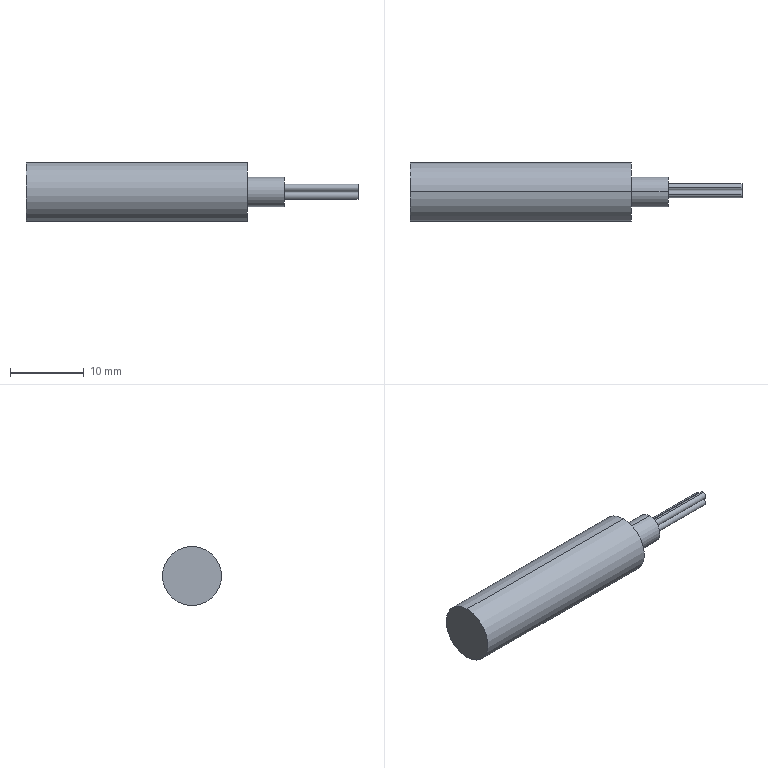Part | STEP file | Sensors | 1 solid | 16 faces | box 45 x 8 x 8 mm | volume 1594 mm3 | cylinder 10 | plane 6 | commonest cylinder face diameters 1 x6 4 x2 8 x2
STEP:
#1=CARTESIAN_POINT('',(34.739,-0.2752,0.03902));
#2=VERTEX_POINT('',#1);
#3=CARTESIAN_POINT('',(34.739,-0.2752,1.039));
#4=VERTEX_POINT('',#3);
#5=CARTESIAN_POINT('',(34.739,-0.2752,0.539));
#6=DIRECTION('',(1.,0.,0.));
#7=DIRECTION('',(0.,0.,-1.));
#8=AXIS2_PLACEMENT_3D('',#5,#6,#7);
#9=CIRCLE('',#8,0.5);
#10=EDGE_CURVE('',#2,#4,#9,.T.);
#11=ORIENTED_EDGE('',*,*,#10,.F.);
#12=CARTESIAN_POINT('',(24.739,-0.2752,0.03902));
#13=VERTEX_POINT('',#12);
#14=CARTESIAN_POINT('',(34.739,-0.2752,0.03902));
#15=DIRECTION('',(-1.,0.,0.));
#16=VECTOR('',#15,1000.);
#17=LINE('',#14,#16);
#18=EDGE_CURVE('',#2,#13,#17,.T.);
#19=ORIENTED_EDGE('',*,*,#18,.T.);
#20=CARTESIAN_POINT('',(24.739,-0.2752,1.039));
#21=VERTEX_POINT('',#20);
#22=CARTESIAN_POINT('',(24.739,-0.2752,0.539));
#23=DIRECTION('',(1.,0.,0.));
#24=DIRECTION('',(0.,0.,-1.));
#25=AXIS2_PLACEMENT_3D('',#22,#23,#24);
#26=CIRCLE('',#25,0.5);
#27=EDGE_CURVE('',#13,#21,#26,.T.);
#28=ORIENTED_EDGE('',*,*,#27,.T.);
#29=CARTESIAN_POINT('',(34.739,-0.2752,1.039));
#30=DIRECTION('',(-1.,0.,0.));
#31=VECTOR('',#30,1000.);
#32=LINE('',#29,#31);
#33=EDGE_CURVE('',#4,#21,#32,.T.);
#34=ORIENTED_EDGE('',*,*,#33,.F.);
#35=EDGE_LOOP('',(#11,#19,#28,#34));
#36=FACE_OUTER_BOUND('',#35,.T.);
#37=CARTESIAN_POINT('',(34.739,-0.2752,0.539));
#38=DIRECTION('',(-1.,0.,0.));
#39=DIRECTION('',(0.,0.,1.));
#40=AXIS2_PLACEMENT_3D('',#37,#38,#39);
#41=CYLINDRICAL_SURFACE('',#40,0.5);
#42=ADVANCED_FACE('',(#36),#41,.T.);
#43=CARTESIAN_POINT('',(34.739,-0.2752,-1.016));
#44=VERTEX_POINT('',#43);
#45=CARTESIAN_POINT('',(34.739,-0.2752,-0.01608));
#46=VERTEX_POINT('',#45);
#47=CARTESIAN_POINT('',(34.739,-0.2752,-0.5161));
#48=DIRECTION('',(1.,0.,0.));
#49=DIRECTION('',(0.,0.,-1.));
#50=AXIS2_PLACEMENT_3D('',#47,#48,#49);
#51=CIRCLE('',#50,0.5);
#52=EDGE_CURVE('',#44,#46,#51,.T.);
#53=ORIENTED_EDGE('',*,*,#52,.F.);
#54=CARTESIAN_POINT('',(24.739,-0.2752,-1.016));
#55=VERTEX_POINT('',#54);
#56=CARTESIAN_POINT('',(34.739,-0.2752,-1.016));
#57=DIRECTION('',(-1.,0.,0.));
#58=VECTOR('',#57,1000.);
#59=LINE('',#56,#58);
#60=EDGE_CURVE('',#44,#55,#59,.T.);
#61=ORIENTED_EDGE('',*,*,#60,.T.);
#62=CARTESIAN_POINT('',(24.739,-0.2752,-0.01608));
#63=VERTEX_POINT('',#62);
#64=CARTESIAN_POINT('',(24.739,-0.2752,-0.5161));
#65=DIRECTION('',(1.,0.,0.));
#66=DIRECTION('',(0.,0.,-1.));
#67=AXIS2_PLACEMENT_3D('',#64,#65,#66);
#68=CIRCLE('',#67,0.5);
#69=EDGE_CURVE('',#55,#63,#68,.T.);
#70=ORIENTED_EDGE('',*,*,#69,.T.);
#71=CARTESIAN_POINT('',(34.739,-0.2752,-0.01608));
#72=DIRECTION('',(-1.,0.,0.));
#73=VECTOR('',#72,1000.);
#74=LINE('',#71,#73);
#75=EDGE_CURVE('',#46,#63,#74,.T.);
#76=ORIENTED_EDGE('',*,*,#75,.F.);
#77=EDGE_LOOP('',(#53,#61,#70,#76));
#78=FACE_OUTER_BOUND('',#77,.T.);
#79=CARTESIAN_POINT('',(34.739,-0.2752,-0.5161));
#80=DIRECTION('',(-1.,0.,0.));
#81=DIRECTION('',(0.,0.,1.));
#82=AXIS2_PLACEMENT_3D('',#79,#80,#81);
#83=CYLINDRICAL_SURFACE('',#82,0.5);
#84=ADVANCED_FACE('',(#78),#83,.T.);
#85=CARTESIAN_POINT('',(34.739,0.6078,-0.5));
#86=VERTEX_POINT('',#85);
#87=CARTESIAN_POINT('',(34.739,0.6078,0.5));
#88=VERTEX_POINT('',#87);
#89=CARTESIAN_POINT('',(34.739,0.6078,0.));
#90=DIRECTION('',(1.,0.,0.));
#91=DIRECTION('',(0.,0.,-1.));
#92=AXIS2_PLACEMENT_3D('',#89,#90,#91);
#93=CIRCLE('',#92,0.5);
#94=EDGE_CURVE('',#86,#88,#93,.T.);
#95=ORIENTED_EDGE('',*,*,#94,.F.);
#96=CARTESIAN_POINT('',(24.739,0.6078,-0.5));
#97=VERTEX_POINT('',#96);
#98=CARTESIAN_POINT('',(34.739,0.6078,-0.5));
#99=DIRECTION('',(-1.,0.,0.));
#100=VECTOR('',#99,1000.);
#101=LINE('',#98,#100);
#102=EDGE_CURVE('',#86,#97,#101,.T.);
#103=ORIENTED_EDGE('',*,*,#102,.T.);
#104=CARTESIAN_POINT('',(24.739,0.6078,0.5));
#105=VERTEX_POINT('',#104);
#106=CARTESIAN_POINT('',(24.739,0.6078,0.));
#107=DIRECTION('',(1.,0.,0.));
#108=DIRECTION('',(0.,0.,-1.));
#109=AXIS2_PLACEMENT_3D('',#106,#107,#108);
#110=CIRCLE('',#109,0.5);
#111=EDGE_CURVE('',#97,#105,#110,.T.);
#112=ORIENTED_EDGE('',*,*,#111,.T.);
#113=CARTESIAN_POINT('',(34.739,0.6078,0.5));
#114=DIRECTION('',(-1.,0.,0.));
#115=VECTOR('',#114,1000.);
#116=LINE('',#113,#115);
#117=EDGE_CURVE('',#88,#105,#116,.T.);
#118=ORIENTED_EDGE('',*,*,#117,.F.);
#119=EDGE_LOOP('',(#95,#103,#112,#118));
#120=FACE_OUTER_BOUND('',#119,.T.);
#121=CARTESIAN_POINT('',(34.739,0.6078,0.));
#122=DIRECTION('',(-1.,0.,0.));
#123=DIRECTION('',(0.,0.,1.));
#124=AXIS2_PLACEMENT_3D('',#121,#122,#123);
#125=CYLINDRICAL_SURFACE('',#124,0.5);
#126=ADVANCED_FACE('',(#120),#125,.T.);
#127=CARTESIAN_POINT('',(24.739,0.,-2.));
#128=VERTEX_POINT('',#127);
#129=CARTESIAN_POINT('',(24.739,0.,2.));
#130=VERTEX_POINT('',#129);
#131=CARTESIAN_POINT('',(24.739,0.,0.));
#132=DIRECTION('',(1.,0.,0.));
#133=DIRECTION('',(0.,0.,-1.));
#134=AXIS2_PLACEMENT_3D('',#131,#132,#133);
#135=CIRCLE('',#134,2.);
#136=EDGE_CURVE('',#128,#130,#135,.T.);
#137=ORIENTED_EDGE('',*,*,#136,.F.);
#138=CARTESIAN_POINT('',(19.739,0.,-2.));
#139=VERTEX_POINT('',#138);
#140=CARTESIAN_POINT('',(24.739,0.,-2.));
#141=DIRECTION('',(-1.,0.,0.));
#142=VECTOR('',#141,1000.);
#143=LINE('',#140,#142);
#144=EDGE_CURVE('',#128,#139,#143,.T.);
#145=ORIENTED_EDGE('',*,*,#144,.T.);
#146=CARTESIAN_POINT('',(19.739,0.,2.));
#147=VERTEX_POINT('',#146);
#148=CARTESIAN_POINT('',(19.739,0.,0.));
#149=DIRECTION('',(1.,0.,0.));
#150=DIRECTION('',(0.,0.,-1.));
#151=AXIS2_PLACEMENT_3D('',#148,#149,#150);
#152=CIRCLE('',#151,2.);
#153=EDGE_CURVE('',#139,#147,#152,.T.);
#154=ORIENTED_EDGE('',*,*,#153,.T.);
#155=CARTESIAN_POINT('',(24.739,0.,2.));
#156=DIRECTION('',(-1.,0.,0.));
#157=VECTOR('',#156,1000.);
#158=LINE('',#155,#157);
#159=EDGE_CURVE('',#130,#147,#158,.T.);
#160=ORIENTED_EDGE('',*,*,#159,.F.);
#161=EDGE_LOOP('',(#137,#145,#154,#160));
#162=FACE_OUTER_BOUND('',#161,.T.);
#163=CARTESIAN_POINT('',(24.739,0.,0.));
#164=DIRECTION('',(-1.,0.,0.));
#165=DIRECTION('',(0.,0.,1.));
#166=AXIS2_PLACEMENT_3D('',#163,#164,#165);
#167=CYLINDRICAL_SURFACE('',#166,2.);
#168=ADVANCED_FACE('',(#162),#167,.T.);
#169=CARTESIAN_POINT('',(19.739,0.,4.));
#170=VERTEX_POINT('',#169);
#171=CARTESIAN_POINT('',(19.739,0.,-4.));
#172=VERTEX_POINT('',#171);
#173=CARTESIAN_POINT('',(19.739,0.,0.));
#174=DIRECTION('',(-1.,0.,0.));
#175=DIRECTION('',(0.,0.,1.));
#176=AXIS2_PLACEMENT_3D('',#173,#174,#175);
#177=CIRCLE('',#176,4.);
#178=EDGE_CURVE('',#170,#172,#177,.T.);
#179=ORIENTED_EDGE('',*,*,#178,.T.);
#180=CARTESIAN_POINT('',(-10.261,0.,-4.));
#181=VERTEX_POINT('',#180);
#182=CARTESIAN_POINT('',(-34.395,0.,-4.));
#183=DIRECTION('',(-1.,0.,0.));
#184=VECTOR('',#183,1000.);
#185=LINE('',#182,#184);
#186=EDGE_CURVE('',#172,#181,#185,.T.);
#187=ORIENTED_EDGE('',*,*,#186,.T.);
#188=CARTESIAN_POINT('',(-10.261,0.,4.));
#189=VERTEX_POINT('',#188);
#190=CARTESIAN_POINT('',(-10.261,0.,0.));
#191=DIRECTION('',(-1.,0.,0.));
#192=DIRECTION('',(0.,0.,1.));
#193=AXIS2_PLACEMENT_3D('',#190,#191,#192);
#194=CIRCLE('',#193,4.);
#195=EDGE_CURVE('',#189,#181,#194,.T.);
#196=ORIENTED_EDGE('',*,*,#195,.F.);
#197=CARTESIAN_POINT('',(-34.395,0.,4.));
#198=DIRECTION('',(-1.,0.,0.));
#199=VECTOR('',#198,1000.);
#200=LINE('',#197,#199);
#201=EDGE_CURVE('',#170,#189,#200,.T.);
#202=ORIENTED_EDGE('',*,*,#201,.F.);
#203=EDGE_LOOP('',(#179,#187,#196,#202));
#204=FACE_OUTER_BOUND('',#203,.T.);
#205=CARTESIAN_POINT('',(-34.395,0.,0.));
#206=DIRECTION('',(-1.,0.,0.));
#207=DIRECTION('',(0.,0.,1.));
#208=AXIS2_PLACEMENT_3D('',#205,#206,#207);
#209=CYLINDRICAL_SURFACE('',#208,4.);
#210=ADVANCED_FACE('',(#204),#209,.T.);
#211=ORIENTED_EDGE('',*,*,#195,.T.);
#212=CARTESIAN_POINT('',(-10.261,0.,0.));
#213=DIRECTION('',(-1.,0.,0.));
#214=DIRECTION('',(0.,0.,1.));
#215=AXIS2_PLACEMENT_3D('',#212,#213,#214);
#216=CIRCLE('',#215,4.);
#217=EDGE_CURVE('',#181,#189,#216,.T.);
#218=ORIENTED_EDGE('',*,*,#217,.T.);
#219=EDGE_LOOP('',(#211,#218));
#220=FACE_OUTER_BOUND('',#219,.T.);
#221=CARTESIAN_POINT('',(-10.261,0.,0.));
#222=DIRECTION('',(1.,0.,0.));
#223=DIRECTION('',(0.,0.,-1.));
#224=AXIS2_PLACEMENT_3D('',#221,#222,#223);
#225=PLANE('',#224);
#226=ADVANCED_FACE('',(#220),#225,.F.);
#227=CARTESIAN_POINT('',(19.739,0.,0.));
#228=DIRECTION('',(1.,0.,0.));
#229=DIRECTION('',(0.,0.,-1.));
#230=AXIS2_PLACEMENT_3D('',#227,#228,#229);
#231=CIRCLE('',#230,2.);
#232=EDGE_CURVE('',#147,#139,#231,.T.);
#233=ORIENTED_EDGE('',*,*,#232,.F.);
#234=ORIENTED_EDGE('',*,*,#153,.F.);
#235=EDGE_LOOP('',(#233,#234));
#236=FACE_BOUND('',#235,.T.);
#237=ORIENTED_EDGE('',*,*,#178,.F.);
#238=CARTESIAN_POINT('',(19.739,0.,0.));
#239=DIRECTION('',(-1.,0.,0.));
#240=DIRECTION('',(0.,0.,1.));
#241=AXIS2_PLACEMENT_3D('',#238,#239,#240);
#242=CIRCLE('',#241,4.);
#243=EDGE_CURVE('',#172,#170,#242,.T.);
#244=ORIENTED_EDGE('',*,*,#243,.F.);
#245=EDGE_LOOP('',(#237,#244));
#246=FACE_OUTER_BOUND('',#245,.T.);
#247=CARTESIAN_POINT('',(19.739,0.,0.));
#248=DIRECTION('',(-1.,0.,0.));
#249=DIRECTION('',(0.,0.,1.));
#250=AXIS2_PLACEMENT_3D('',#247,#248,#249);
#251=PLANE('',#250);
#252=ADVANCED_FACE('',(#236,#246),#251,.F.);
#253=ORIENTED_EDGE('',*,*,#186,.F.);
#254=ORIENTED_EDGE('',*,*,#243,.T.);
#255=ORIENTED_EDGE('',*,*,#201,.T.);
#256=ORIENTED_EDGE('',*,*,#217,.F.);
#257=EDGE_LOOP('',(#253,#254,#255,#256));
#258=FACE_OUTER_BOUND('',#257,.T.);
#259=CARTESIAN_POINT('',(-34.395,0.,0.));
#260=DIRECTION('',(-1.,0.,0.));
#261=DIRECTION('',(0.,0.,1.));
#262=AXIS2_PLACEMENT_3D('',#259,#260,#261);
#263=CYLINDRICAL_SURFACE('',#262,4.);
#264=ADVANCED_FACE('',(#258),#263,.T.);
#265=ORIENTED_EDGE('',*,*,#144,.F.);
#266=CARTESIAN_POINT('',(24.739,0.,0.));
#267=DIRECTION('',(1.,0.,0.));
#268=DIRECTION('',(0.,0.,-1.));
#269=AXIS2_PLACEMENT_3D('',#266,#267,#268);
#270=CIRCLE('',#269,2.);
#271=EDGE_CURVE('',#130,#128,#270,.T.);
#272=ORIENTED_EDGE('',*,*,#271,.F.);
#273=ORIENTED_EDGE('',*,*,#159,.T.);
#274=ORIENTED_EDGE('',*,*,#232,.T.);
#275=EDGE_LOOP('',(#265,#272,#273,#274));
#276=FACE_OUTER_BOUND('',#275,.T.);
#277=CARTESIAN_POINT('',(24.739,0.,0.));
#278=DIRECTION('',(-1.,0.,0.));
#279=DIRECTION('',(0.,0.,1.));
#280=AXIS2_PLACEMENT_3D('',#277,#278,#279);
#281=CYLINDRICAL_SURFACE('',#280,2.);
#282=ADVANCED_FACE('',(#276),#281,.T.);
#283=CARTESIAN_POINT('',(24.739,-0.2752,0.539));
#284=DIRECTION('',(1.,0.,0.));
#285=DIRECTION('',(0.,0.,-1.));
#286=AXIS2_PLACEMENT_3D('',#283,#284,#285);
#287=CIRCLE('',#286,0.5);
#288=EDGE_CURVE('',#21,#13,#287,.T.);
#289=ORIENTED_EDGE('',*,*,#288,.F.);
#290=ORIENTED_EDGE('',*,*,#27,.F.);
#291=EDGE_LOOP('',(#289,#290));
#292=FACE_BOUND('',#291,.T.);
#293=CARTESIAN_POINT('',(24.739,-0.2752,-0.5161));
#294=DIRECTION('',(1.,0.,0.));
#295=DIRECTION('',(0.,0.,-1.));
#296=AXIS2_PLACEMENT_3D('',#293,#294,#295);
#297=CIRCLE('',#296,0.5);
#298=EDGE_CURVE('',#63,#55,#297,.T.);
#299=ORIENTED_EDGE('',*,*,#298,.F.);
#300=ORIENTED_EDGE('',*,*,#69,.F.);
#301=EDGE_LOOP('',(#299,#300));
#302=FACE_BOUND('',#301,.T.);
#303=CARTESIAN_POINT('',(24.739,0.6078,0.));
#304=DIRECTION('',(1.,0.,0.));
#305=DIRECTION('',(0.,0.,-1.));
#306=AXIS2_PLACEMENT_3D('',#303,#304,#305);
#307=CIRCLE('',#306,0.5);
#308=EDGE_CURVE('',#105,#97,#307,.T.);
#309=ORIENTED_EDGE('',*,*,#308,.F.);
#310=ORIENTED_EDGE('',*,*,#111,.F.);
#311=EDGE_LOOP('',(#309,#310));
#312=FACE_BOUND('',#311,.T.);
#313=ORIENTED_EDGE('',*,*,#271,.T.);
#314=ORIENTED_EDGE('',*,*,#136,.T.);
#315=EDGE_LOOP('',(#313,#314));
#316=FACE_OUTER_BOUND('',#315,.T.);
#317=CARTESIAN_POINT('',(24.739,0.,0.));
#318=DIRECTION('',(1.,0.,0.));
#319=DIRECTION('',(0.,0.,-1.));
#320=AXIS2_PLACEMENT_3D('',#317,#318,#319);
#321=PLANE('',#320);
#322=ADVANCED_FACE('',(#292,#302,#312,#316),#321,.T.);
#323=ORIENTED_EDGE('',*,*,#102,.F.);
#324=CARTESIAN_POINT('',(34.739,0.6078,0.));
#325=DIRECTION('',(1.,0.,0.));
#326=DIRECTION('',(0.,0.,-1.));
#327=AXIS2_PLACEMENT_3D('',#324,#325,#326);
#328=CIRCLE('',#327,0.5);
#329=EDGE_CURVE('',#88,#86,#328,.T.);
#330=ORIENTED_EDGE('',*,*,#329,.F.);
#331=ORIENTED_EDGE('',*,*,#117,.T.);
#332=ORIENTED_EDGE('',*,*,#308,.T.);
#333=EDGE_LOOP('',(#323,#330,#331,#332));
#334=FACE_OUTER_BOUND('',#333,.T.);
#335=CARTESIAN_POINT('',(34.739,0.6078,0.));
#336=DIRECTION('',(-1.,0.,0.));
#337=DIRECTION('',(0.,0.,1.));
#338=AXIS2_PLACEMENT_3D('',#335,#336,#337);
#339=CYLINDRICAL_SURFACE('',#338,0.5);
#340=ADVANCED_FACE('',(#334),#339,.T.);
#341=ORIENTED_EDGE('',*,*,#329,.T.);
#342=ORIENTED_EDGE('',*,*,#94,.T.);
#343=EDGE_LOOP('',(#341,#342));
#344=FACE_OUTER_BOUND('',#343,.T.);
#345=CARTESIAN_POINT('',(34.739,0.6078,0.));
#346=DIRECTION('',(1.,0.,0.));
#347=DIRECTION('',(0.,0.,-1.));
#348=AXIS2_PLACEMENT_3D('',#345,#346,#347);
#349=PLANE('',#348);
#350=ADVANCED_FACE('',(#344),#349,.T.);
#351=ORIENTED_EDGE('',*,*,#60,.F.);
#352=CARTESIAN_POINT('',(34.739,-0.2752,-0.5161));
#353=DIRECTION('',(1.,0.,0.));
#354=DIRECTION('',(0.,0.,-1.));
#355=AXIS2_PLACEMENT_3D('',#352,#353,#354);
#356=CIRCLE('',#355,0.5);
#357=EDGE_CURVE('',#46,#44,#356,.T.);
#358=ORIENTED_EDGE('',*,*,#357,.F.);
#359=ORIENTED_EDGE('',*,*,#75,.T.);
#360=ORIENTED_EDGE('',*,*,#298,.T.);
#361=EDGE_LOOP('',(#351,#358,#359,#360));
#362=FACE_OUTER_BOUND('',#361,.T.);
#363=CARTESIAN_POINT('',(34.739,-0.2752,-0.5161));
#364=DIRECTION('',(-1.,0.,0.));
#365=DIRECTION('',(0.,0.,1.));
#366=AXIS2_PLACEMENT_3D('',#363,#364,#365);
#367=CYLINDRICAL_SURFACE('',#366,0.5);
#368=ADVANCED_FACE('',(#362),#367,.T.);
#369=ORIENTED_EDGE('',*,*,#357,.T.);
#370=ORIENTED_EDGE('',*,*,#52,.T.);
#371=EDGE_LOOP('',(#369,#370));
#372=FACE_OUTER_BOUND('',#371,.T.);
#373=CARTESIAN_POINT('',(34.739,-0.2752,-0.5161));
#374=DIRECTION('',(1.,0.,0.));
#375=DIRECTION('',(0.,0.,-1.));
#376=AXIS2_PLACEMENT_3D('',#373,#374,#375);
#377=PLANE('',#376);
#378=ADVANCED_FACE('',(#372),#377,.T.);
#379=ORIENTED_EDGE('',*,*,#18,.F.);
#380=CARTESIAN_POINT('',(34.739,-0.2752,0.539));
#381=DIRECTION('',(1.,0.,0.));
#382=DIRECTION('',(0.,0.,-1.));
#383=AXIS2_PLACEMENT_3D('',#380,#381,#382);
#384=CIRCLE('',#383,0.5);
#385=EDGE_CURVE('',#4,#2,#384,.T.);
#386=ORIENTED_EDGE('',*,*,#385,.F.);
#387=ORIENTED_EDGE('',*,*,#33,.T.);
#388=ORIENTED_EDGE('',*,*,#288,.T.);
#389=EDGE_LOOP('',(#379,#386,#387,#388));
#390=FACE_OUTER_BOUND('',#389,.T.);
#391=CARTESIAN_POINT('',(34.739,-0.2752,0.539));
#392=DIRECTION('',(-1.,0.,0.));
#393=DIRECTION('',(0.,0.,1.));
#394=AXIS2_PLACEMENT_3D('',#391,#392,#393);
#395=CYLINDRICAL_SURFACE('',#394,0.5);
#396=ADVANCED_FACE('',(#390),#395,.T.);
#397=ORIENTED_EDGE('',*,*,#385,.T.);
#398=ORIENTED_EDGE('',*,*,#10,.T.);
#399=EDGE_LOOP('',(#397,#398));
#400=FACE_OUTER_BOUND('',#399,.T.);
#401=CARTESIAN_POINT('',(34.739,-0.2752,0.539));
#402=DIRECTION('',(1.,0.,0.));
#403=DIRECTION('',(0.,0.,-1.));
#404=AXIS2_PLACEMENT_3D('',#401,#402,#403);
#405=PLANE('',#404);
#406=ADVANCED_FACE('',(#400),#405,.T.);
#407=CLOSED_SHELL('',(#42,#84,#126,#168,#210,#226,#252,#264,#282,#322,#340,#350,#368,#378,#396,#406));
#408=MANIFOLD_SOLID_BREP('',#407);
#409=CARTESIAN_POINT('',(0.,0.,0.));
#410=DIRECTION('',(0.,0.,1.));
#411=DIRECTION('',(1.,0.,0.));
#412=AXIS2_PLACEMENT_3D('',#409,#410,#411);
#413=(LENGTH_UNIT()NAMED_UNIT(*)SI_UNIT(.MILLI.,.METRE.));
#414=UNCERTAINTY_MEASURE_WITH_UNIT(LENGTH_MEASURE(0.00001),#413,'','');
#415=(NAMED_UNIT(*)PLANE_ANGLE_UNIT()SI_UNIT($,.RADIAN.));
#416=(NAMED_UNIT(*)SI_UNIT($,.STERADIAN.)SOLID_ANGLE_UNIT());
#417=(GEOMETRIC_REPRESENTATION_CONTEXT(3)GLOBAL_UNCERTAINTY_ASSIGNED_CONTEXT((#414))GLOBAL_UNIT_ASSIGNED_CONTEXT((#413,#415,#416))REPRESENTATION_CONTEXT('',''));
#418=ADVANCED_BREP_SHAPE_REPRESENTATION('',(#408,#412),#417);